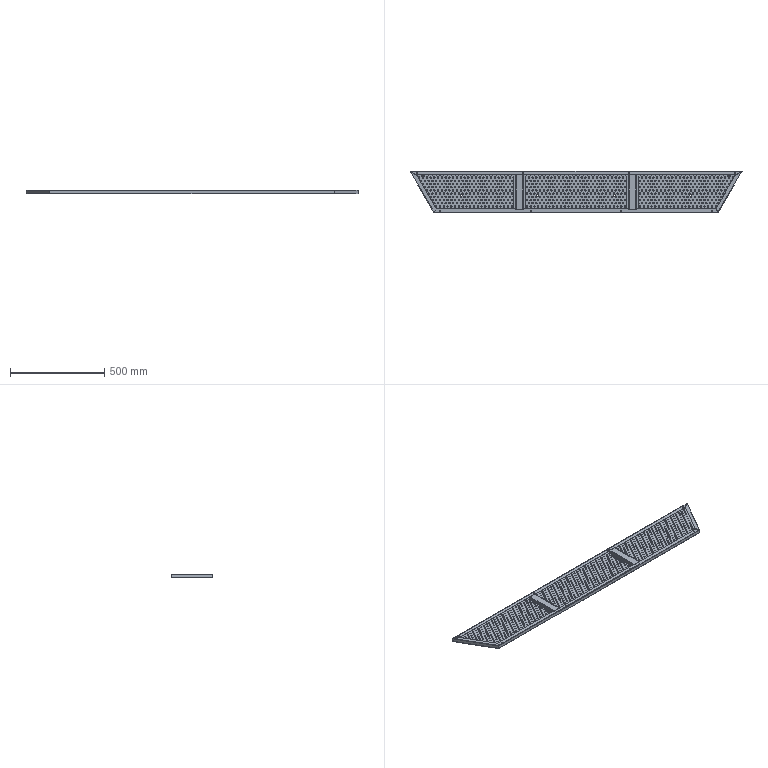Part | SolidWorks | features LocalLPattern 1, ReferencePattern 1 | 3 solids | 2141 faces | box 1758 x 220 x 20 mm | volume 727420 mm3 | cylinder 1974 | plane 148 | spline 19 | commonest cylinder face diameters 7.2 x1908 6 x18 6.4 x16 1 x8 2 x8 4 x8